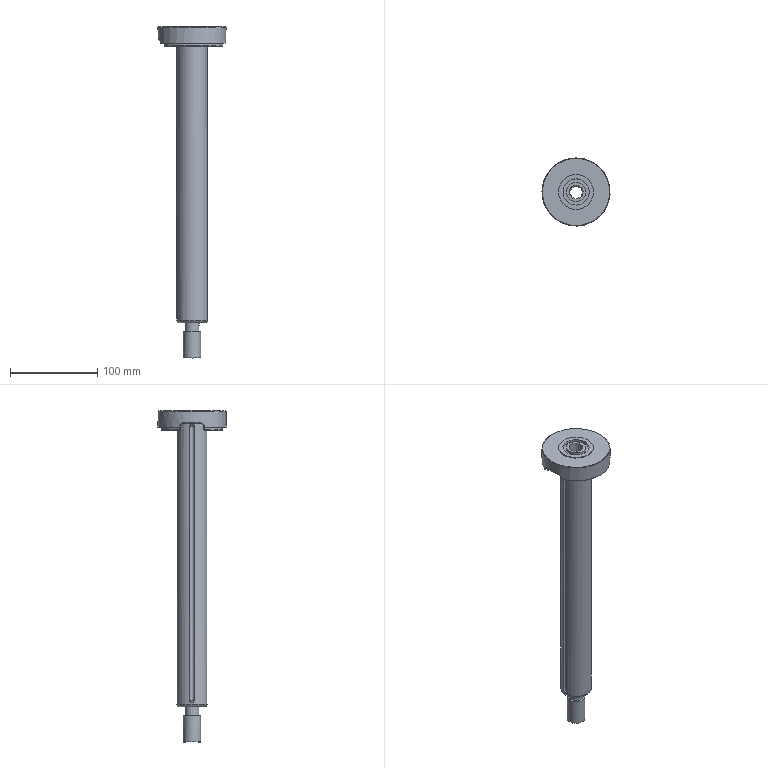Part | STEP file | solid 189 | 1 solid | 52 faces | box 78 x 78 x 380.197 mm | volume 321503 mm3 | plane 21 | cylinder 15 | spline 8 | cone 5 | sphere 2 | torus 1 | commonest cylinder face diameters 5 x3 10 x2 16 x2 14 x1 20 x1 22 x1